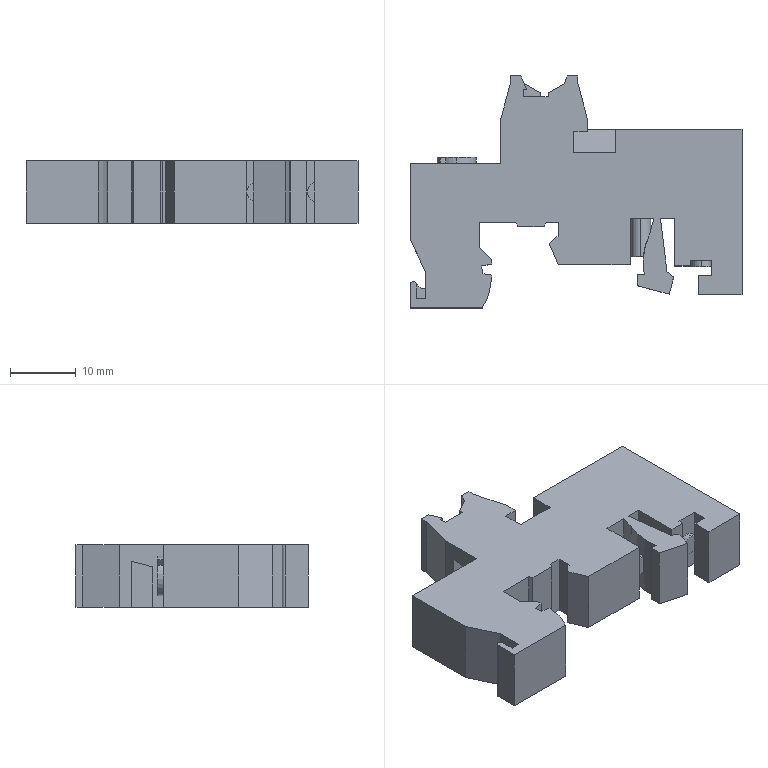Part | STEP file | End clamp-E UK-1201442 | 1 solid | 114 faces | box 50.5 x 35.3 x 9.5 mm | volume 9735 mm3 | plane 97 | cylinder 17 | commonest cylinder face diameters 6 x9 3 x4 1 x1 2 x1 19 x1 20 x1